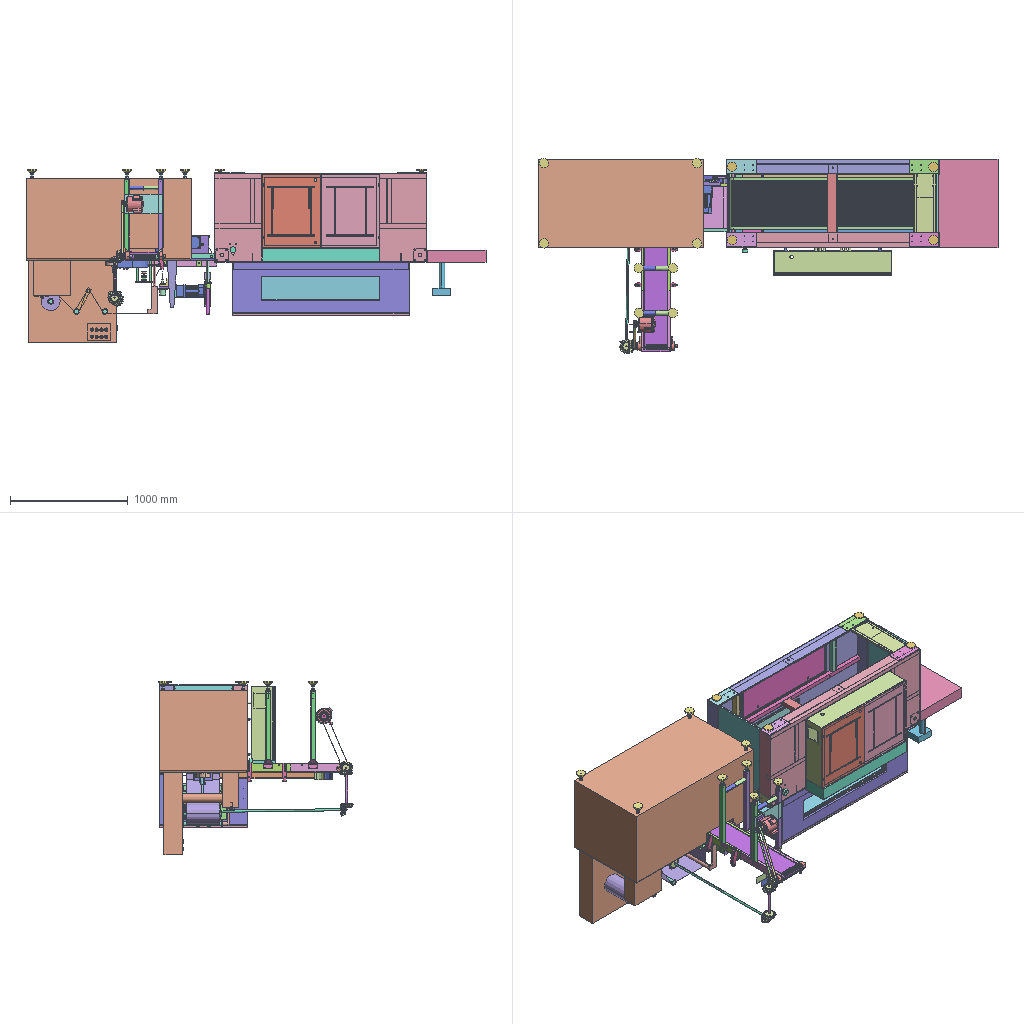Assembly | STEP file | 127 different items | 196 placed | box 3903 x 1652 x 1470 mm
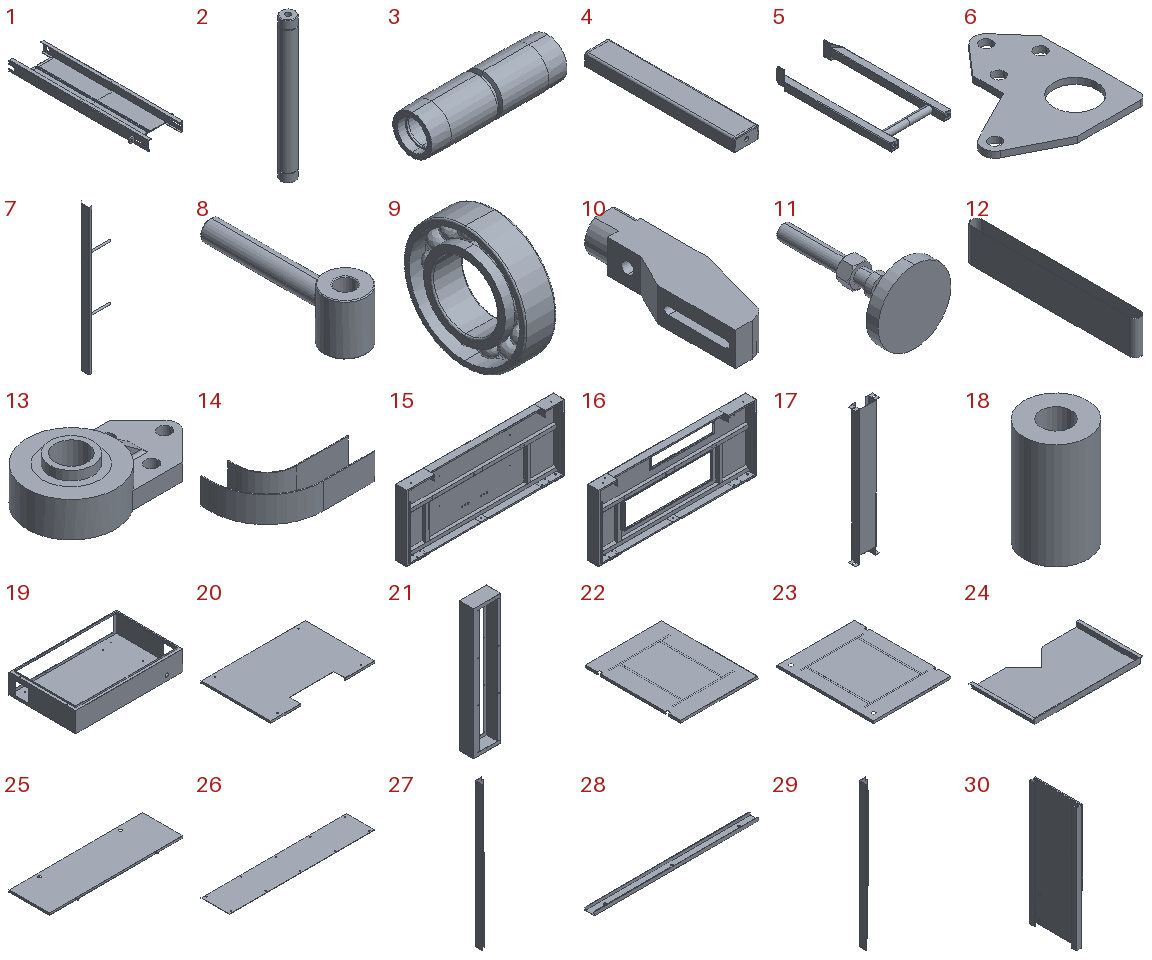Parts list (item | name | quantity | parent item | size | volume):
1 | MM-P41130-01_1 | x1 | - | 314 x 1000 x 70 mm | 800616 mm3
2 | MM-P46715-03_1 | x1 | - | 25 x 25 x 246 mm | 117700 mm3
3 | MM-P46715-04_1 | x1 | - | 215 x 64 x 64 mm | 333247 mm3
4 | MM-P46715-05_1 | x2 | - | 40 x 245 x 20 mm | 40958 mm3
5 | MM-P46715-07_1 | x2 | - | 334.243 x 661.5 x 80 mm | 460101 mm3
6 | MM-P46715-11_1 | x1 | - | 103 x 112 x 5 mm | 30189 mm3
7 | MM-P41130-12_1 | x2 | - | 151.5 x 53.167 x 800 mm | 109265 mm3
8 | M10-120_1 | x2 | - | 25 x 92.5 x 30 mm | 19534 mm3
9 | 6005-2Z_1 | x2 | - | 12 x 47 x 47 mm | 9163 mm3
10 | - | x4 | - | 44.5 x 151 x 30 mm | 132729 mm3
11 | - | x8 | - | 80 x 144 x 80 mm | 131101 mm3
12 | MM-P41130-13_1 | x1 | - | 67 x 999.5 x 200 mm | 621232 mm3
13 | UCFB205_1 | x2 | - | 116 x 68 x 34 mm | 110392 mm3
14 | - | x1 | - | 252 x 152 x 60 mm | 71299 mm3
15 | - | x1 | - | 1800 x 145 x 755 mm | 5256962 mm3
16 | - | x1 | - | 1800 x 145 x 755 mm | 4684441 mm3
17 | - | x1 | - | 120 x 40 x 664 mm | 146043 mm3
18 | - | x4 | - | 18 x 18 x 30 mm | 5932 mm3
19 | - | x1 | - | 1000 x 625 x 230.5 mm | 1788128 mm3
20 | - | x1 | - | 750 x 500 x 15 mm | 567742 mm3
21 | - | x1 | - | 210 x 110 x 1000 mm | 594029 mm3
22 | - | x1 | - | 508 x 622 x 18 mm | 582197 mm3
23 | - | x1 | - | 498 x 622 x 16 mm | 475643 mm3
24 | - | x1 | - | 316 x 180 x 15 mm | 94868 mm3
25 | - | x1 | - | 998 x 313 x 16 mm | 527029 mm3
26 | - | x1 | - | 718 x 138 x 1.5 mm | 148331 mm3
27 | - | x1 | - | 73.2 x 96 x 1315 mm | 258859 mm3
28 | - | x2 | - | 492 x 27 x 10 mm | 32318 mm3
29 | - | x1 | - | 73.2 x 96 x 1315 mm | 258859 mm3
30 | - | x1 | - | 25 x 190 x 500 mm | 670860 mm3
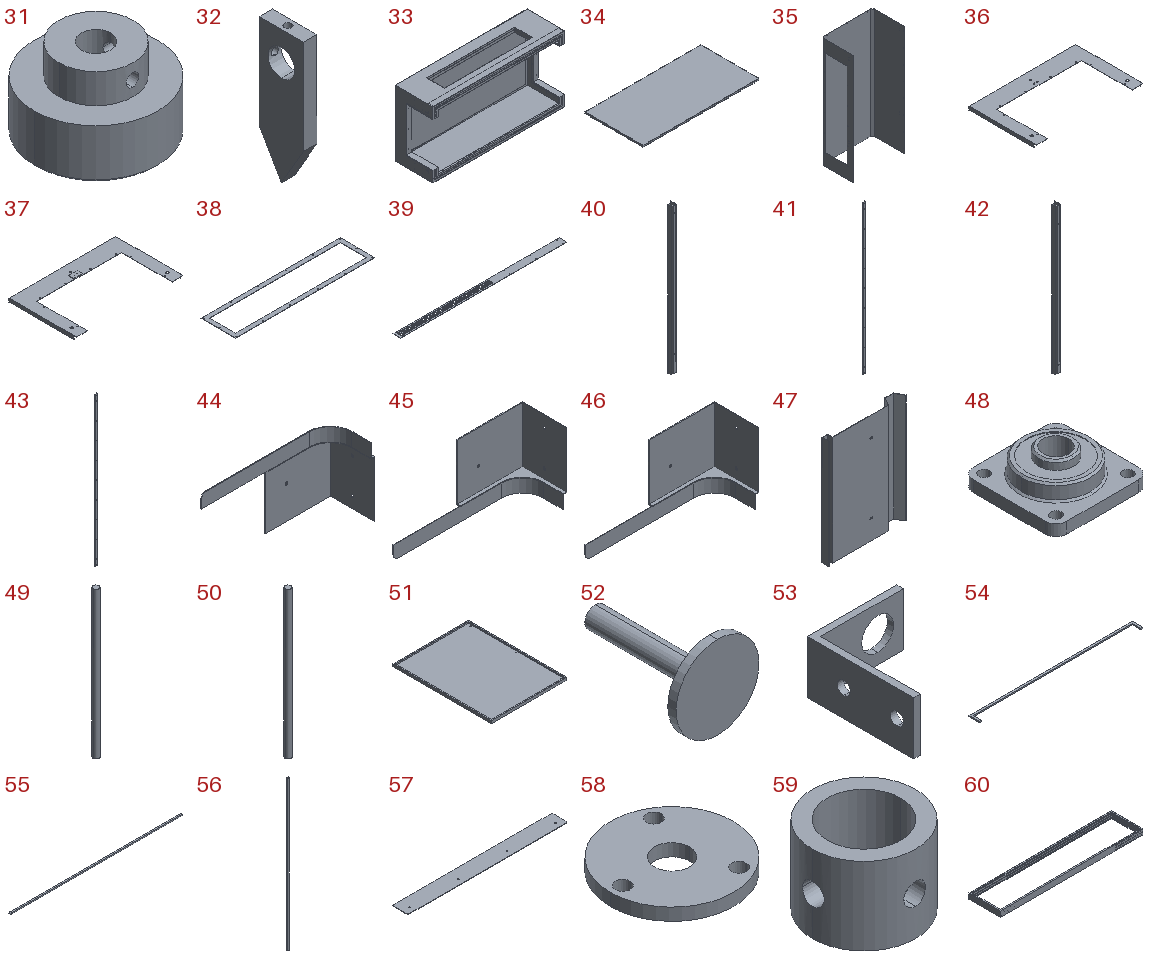31 | - | x1 | - | 50 x 50 x 32 mm | 44461 mm3
32 | - | x1 | - | 6 x 20 x 60 mm | 5382 mm3
33 | - | x1 | - | 1500 x 430 x 750 mm | 6110205 mm3
34 | - | x1 | - | 1500 x 750 x 20 mm | 1901997 mm3
35 | - | x1 | - | 628 x 396 x 1370 mm | 1949197 mm3
36 | - | x1 | - | 632 x 399.5 x 22.5 mm | 152413 mm3
37 | - | x1 | - | 632 x 399.5 x 23 mm | 156800 mm3
38 | - | x1 | - | 1064 x 264 x 2 mm | 161000 mm3
39 | - | x2 | - | 1280 x 60 x 1.5 mm | 89815 mm3
40 | - | x1 | - | 51.2 x 55 x 1530 mm | 316686 mm3
41 | - | x1 | - | 20 x 8 x 1620 mm | 65186 mm3
42 | - | x1 | - | 51.2 x 55 x 1530 mm | 316686 mm3
43 | - | x1 | - | 20 x 8 x 1620 mm | 65186 mm3
44 | - | x2 | - | 301.5 x 102 x 158 mm | 67738 mm3
45 | - | x1 | - | 301.5 x 102 x 158 mm | 67738 mm3
46 | - | x1 | - | 301.5 x 102 x 158 mm | 67738 mm3
47 | - | x1 | - | 281.999 x 34.5 x 390 mm | 208043 mm3
48 | UCF206_1 | x4 | - | 108 x 108 x 40.2 mm | 215781 mm3
49 | - | x1 | - | 30 x 30 x 742 mm | 519728 mm3
50 | - | x1 | - | 30 x 30 x 742 mm | 521298 mm3
51 | - | x2 | - | 498 x 650 x 17.5 mm | 560596 mm3
52 | - | x4 | - | 80 x 118 x 80 mm | 97023 mm3
53 | - | x4 | - | 42 x 50 x 25 mm | 5975 mm3
54 | - | x2 | - | 1458 x 94 x 10 mm | 289800 mm3
55 | - | x2 | - | 1620 x 17.6 x 10 mm | 284365 mm3
56 | - | x2 | - | 14 x 14 x 1400 mm | 203252 mm3
57 | - | x2 | - | 820 x 80 x 2 mm | 130931 mm3
58 | - | x2 | - | 50 x 50 x 5 mm | 8602 mm3
59 | - | x4 | - | 20 x 20 x 15 mm | 2256 mm3
60 | - | x1 | - | 1025 x 225 x 40 mm | 726960 mm3
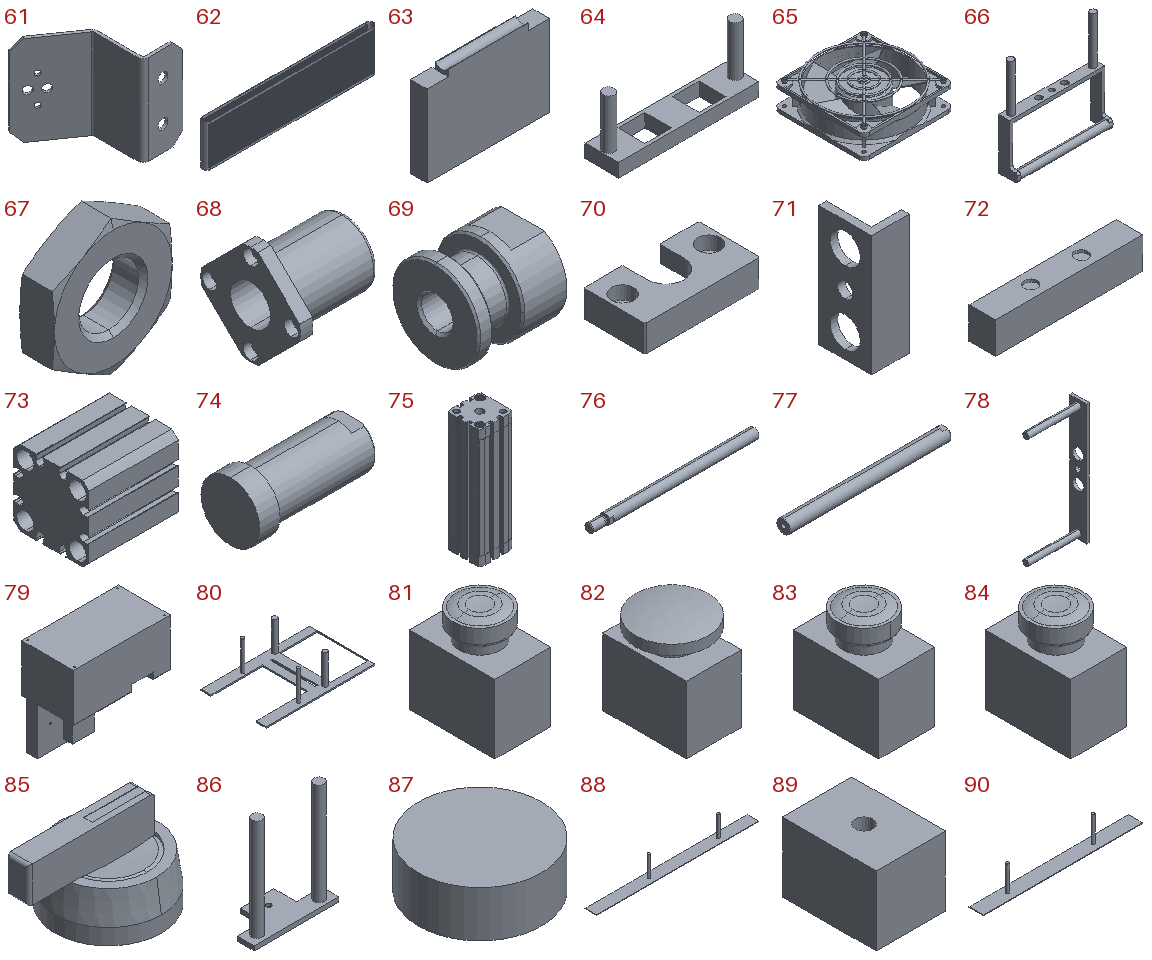61 | - | x1 | - | 44.575 x 43.436 x 45 mm | 4767 mm3
62 | - | x1 | - | 1763 x 82 x 434 mm | 1814355 mm3
63 | - | x1 | - | 750 x 100 x 540 mm | 33368808 mm3
64 | - | x1 | - | 620 x 150 x 280 mm | 4744618 mm3
65 | - | x2 | - | 122 x 122 x 36 mm | 116866 mm3
66 | - | x1 | in 214048b-01-45-00_asm_1 | 440 x 88 x 456 mm | 1386399 mm3
67 | HI_DIN-439-B - M10x1.25(F)_9-a_1_2 | x2 | in ADN-40-150-A-P-A-a_1_2, ADN-40-150-A-P-A-a_1-1_1 | 17 x 5 x 19.63 mm | 939.612 mm3
68 | LHFSF25-2.15-02-02-a_2 | x4 | in 216059B-02-40-00_2 | 59 x 62 x 62 mm | 52716 mm3
69 | FJCL10-1_25-8-a_2 | x2 | in 216059B-02-40-00_2 | 24 x 24 x 24 mm | 7197 mm3
70 | HLRA16-a_2 | x2 | in 216059B-02-40-00_2 | 56 x 30 x 13 mm | 14203 mm3
71 | - | x1 | in 216059B-02-40-00_2 | 50 x 70 x 160 mm | 147726 mm3
72 | - | x2 | in 216059B-02-40-00_2 | 280 x 50 x 60 mm | 835091 mm3
73 | _MSCCN25-15_c_1 | x1 | in MSCCN25-15_1 | 47.5 x 40 x 40 mm | 56452 mm3
74 | _MSCCN25-15_rod_1 | x1 | in MSCCN25-15_1 | 30 x 14.4 x 14.4 mm | 3377 mm3
75 | HI_536288 ADN-150P-----(Z)_1-a_1_1 | x1 | in ADN-40-150-A-P-A-a_1-1_1 | 54.5 x 54.5 x 195 mm | 304101 mm3
76 | HI_536288 ADN-150P0----(KS)_1-a_1_2 | x1 | in ADN-40-150-A-P-A-a_1-1_1 | 193.7 x 12 x 12 mm | 21128 mm3
77 | VFJC25-300-M10-SC290-qwwq-a_2 | x2 | - | 300 x 25 x 25 mm | 145438 mm3
78 | - | x1 | - | 200 x 60 x 440 mm | 380176 mm3
79 | - | x1 | - | 1400 x 750 x 1396 mm | 760190191 mm3
80 | - | x1 | - | 800 x 480 x 230 mm | 2020030 mm3
81 | ZBE-101-Y-1_1 | x1 | - | 30 x 46 x 53.196 mm | 59289 mm3
82 | ZBE-101-STOP-1_1 | x2 | - | 40 x 46 x 52.3 mm | 62411 mm3
83 | ZBE-101-R-1_1 | x1 | - | 30 x 46 x 53.196 mm | 59289 mm3
84 | ZBE-101-G-1_1 | x7 | - | 30 x 46 x 53.196 mm | 59289 mm3
85 | LAY8_1-1_1 | x1 | - | 39.873 x 29.5 x 22.9 mm | 10327 mm3
86 | - | x1 | - | 150 x 70 x 188 mm | 146525 mm3
87 | - | x1 | - | 40 x 40 x 23 mm | 20263 mm3
88 | - | x1 | - | 700 x 50 x 93 mm | 84294 mm3
89 | - | x4 | - | 40 x 54 x 40 mm | 83258 mm3
90 | - | x1 | - | 560 x 50 x 93 mm | 70294 mm3
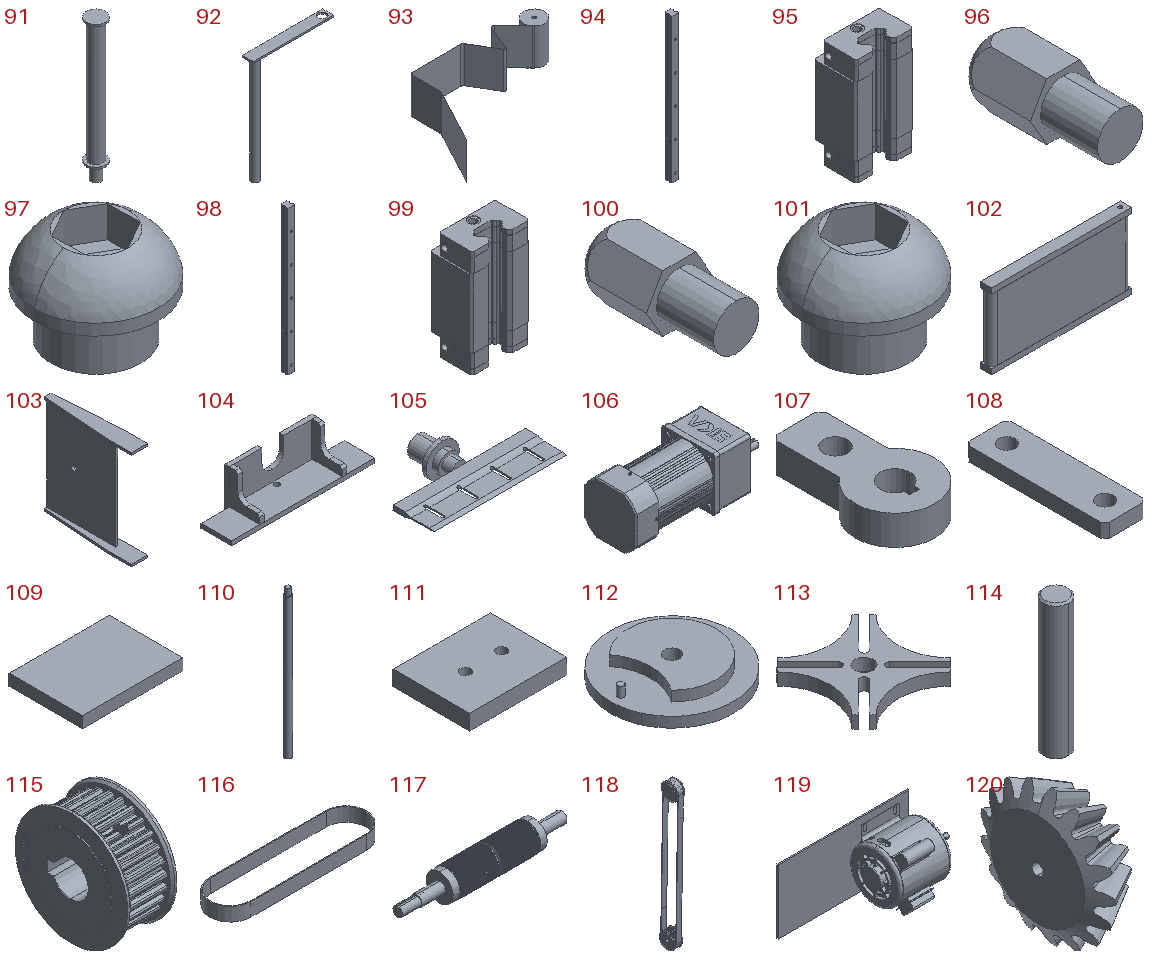91 | JUANZHOU_1 | x3 | - | 50 x 50 x 370 mm | 364990 mm3
92 | - | x1 | - | 240 x 32 x 325 mm | 157588 mm3
93 | - | x1 | - | 1160 x 667.187 x 280 mm | 5746946 mm3
94 | - | x1 | - | 15 x 15 x 300 mm | 55463 mm3
95 | - | x1 | - | 34 x 23.7 x 61.4 mm | 36598 mm3
96 | - | x1 | - | 5.774 x 12.16 x 5 mm | 199.597 mm3
97 | - | x1 | - | 5.5 x 5.5 x 4.2 mm | 58.227 mm3
98 | - | x1 | - | 15 x 15 x 300 mm | 55463 mm3
99 | - | x1 | - | 34 x 23.7 x 61.4 mm | 36598 mm3
100 | - | x1 | - | 5.774 x 12.16 x 5 mm | 199.597 mm3
101 | - | x1 | - | 5.5 x 5.5 x 4.2 mm | 58.227 mm3
102 | - | x1 | - | 760 x 60 x 410 mm | 18296796 mm3
103 | - | x1 | - | 70 x 400 x 430 mm | 1666858 mm3
104 | - | x1 | - | 330 x 80 x 90 mm | 438268 mm3
105 | - | x1 | - | 320 x 200 x 80 mm | 390081 mm3
106 | - | x2 | - | 277 x 108.652 x 108.652 mm | 2253105 mm3
107 | - | x1 | - | 40 x 70 x 15 mm | 25956 mm3
108 | - | x1 | - | 30 x 100 x 10 mm | 27558 mm3
109 | - | x1 | - | 150 x 110 x 17 mm | 280500 mm3
110 | - | x1 | - | 20 x 20 x 460 mm | 141681 mm3
111 | - | x1 | - | 190 x 150 x 30 mm | 836150 mm3
112 | - | x1 | - | 120 x 120 x 20 mm | 158754 mm3
113 | - | x1 | - | 79.917 x 79.917 x 10 mm | 31022 mm3
114 | - | x1 | - | 15 x 15 x 80 mm | 14092 mm3
115 | - | x2 | - | 22 x 48 x 48 mm | 27125 mm3
116 | - | x1 | - | 173.39 x 45.75 x 15 mm | 5938 mm3
117 | MM-P46715-02_1 | x1 | in Modified main assembly | 375.959 x 63.996 x 63.999 mm | 524542 mm3
118 | _X2_51434EF6_X0_21_1 | x1 | in Modified main assembly | 29.173 x 69.582 x 540.649 mm | 150138 mm3
119 | _X2_51434EF6_X0_22_1 | x1 | in Modified main assembly | 358.567 x 145.946 x 163 mm | 1839939 mm3
120 | Bevel gear 17×2 | x6 | in Modified main assembly | 38.391 x 112.113 x 112.556 mm | 206962 mm3
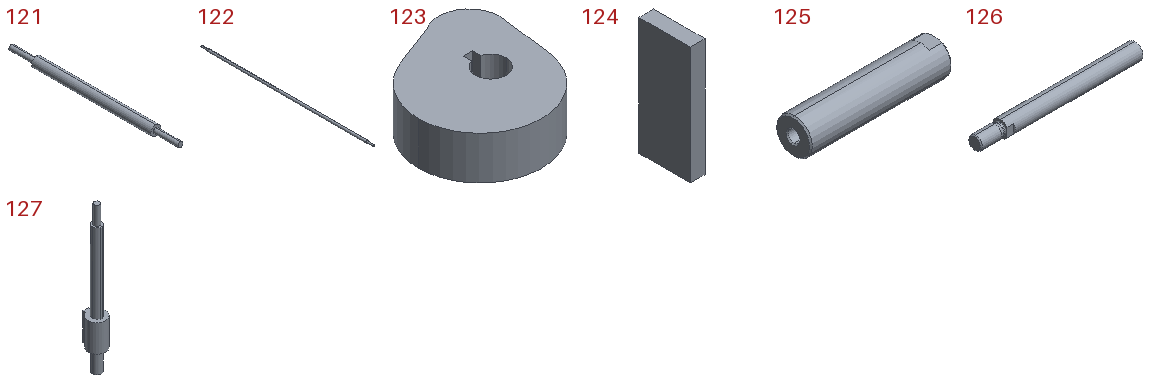121 | Fixed long shaft | x1 | in Modified main assembly | 19.77 x 340 x 19.77 mm | 81528 mm3
122 | Bevel gear fixed shaft | x1 | in Modified main assembly | 18 x 1200 x 18 mm | 287770 mm3
123 | Disc cam | x1 | in Modified main assembly | 105.129 x 114.018 x 35 mm | 298782 mm3
124 | Part 1 | x1 | in Modified main assembly | 20 x 70 x 160 mm | 224000 mm3
125 | Part 2 | x2 | in Modified main assembly | 100 x 25 x 25 mm | 47263 mm3
126 | Part 4 | x1 | in Modified main assembly | 119 x 12 x 12 mm | 12679 mm3
127 | Camshaft | x1 | in Modified main assembly | 38.228 x 43.828 x 320 mm | 147567 mm3
Placements (level | parent | child | x y z in mm | rotation matrix by rows):
1 | Modified main assembly | subassembly 2 | -1135.176 -5611.395 2452.198 | 1 0 0 0 1 0 0 0 1
2 | subassembly 2 | MM-P41130-01_1 | 910.011 5927.051 -736.46 | -1 0 0 0 -1 0 0 0 1
2 | subassembly 2 | MM-P46715-03_1 | 910.011 6389.551 -736.5 | 0 0 1 -0.5368 -0.8437 0 0.8437 -0.5368 0
2 | subassembly 2 | MM-P46715-04_1 | 910.011 6389.551 -736.5 | -1 0 0 0 0.8554 -0.5179 0 -0.5179 -0.8554
2 | subassembly 2 | MM-P46715-05_1 | 910.011 5427.051 -721.5 | 0 1 0 1 0 0 0 0 -1
2 | subassembly 2 | MM-P46715-05_1 | 910.011 6427.051 -721.5 | 0 1 0 1 0 0 0 0 -1
2 | subassembly 2 | MM-P46715-07_1 | 910.011 5737.051 -80.0 | -1 0 0 0 0 -1 0 -1 -0
2 | subassembly 2 | MM-P46715-07_1 | 910.011 6117.051 -80.0 | -1 0 0 0 0 -1 0 -1 0
2 | subassembly 2 | MM-P46715-11_1 | 1040.011 5457.051 -736.5 | 0 0 -1 0 1 0 1 0 0
2 | subassembly 2 | MM-P41130-12_1 | 878.511 6127.051 -825.0 | -1 0 0 0 0 -1 0 -1 0
2 | subassembly 2 | MM-P41130-12_1 | 941.511 6127.051 -825.0 | 1 0 0 0 0 1 0 -1 -0
2 | subassembly 2 | M10-120_1 | 785.011 6389.551 -736.5 | 0 0 -1 0 -1 0 -1 0 -0
2 | subassembly 2 | M10-120_1 | 1067.373 6389.551 -736.5 | 0 0 -1 0 -1 0 -1 0 -0
2 | subassembly 2 | 6005-2Z_1 | 808.511 6389.551 -736.5 | -1 0 0 0 -0.2495 0.9684 0 0.9684 0.2495
2 | subassembly 2 | 6005-2Z_1 | 1011.511 6389.551 -736.5 | -1 0 0 0 -0.2495 0.9684 0 0.9684 0.2495
2 | subassembly 2 | subassembly 3 | 762.761 6277.051 -772.0 | -1 0 0 0 0 -1 0 -1 0
2 | subassembly 2 | subassembly 4 | 1055.011 5737.051 -0.0 | 0.1728 0 0.985 -0.985 0 0.1728 0 -1 -0
2 | subassembly 2 | subassembly 4 | 1055.011 6117.051 -0.0 | 0.2654 0 0.9641 -0.9641 0 0.2654 0 -1 -0
2 | subassembly 2 | subassembly 4 | 765.011 6117.051 -0.0 | -0.5406 0 -0.8413 0.8413 0 -0.5406 0 -1 -0
2 | subassembly 2 | subassembly 4 | 765.011 5737.051 -0.0 | -0.8402 0 -0.5422 0.5422 0 -0.8402 0 -1 -0
2 | subassembly 2 | subassembly 3 | 1057.261 6277.051 -772.0 | 1 0 0 0 0 1 0 -1 -0
2 | subassembly 2 | MM-P41130-13_1 | 910.011 6404.551 -720 | 0 0 1 0 1 0 -1 0 0
2 | subassembly 2 | subassembly 3 | 762.761 5977.051 -772.0 | -1 0 0 0 0 -1 0 -1 0
2 | subassembly 2 | subassembly 3 | 1057.261 5977.051 -772.0 | 1 0 0 0 0 1 0 -1 0
2 | subassembly 2 | UCFB205_1 | 1040.011 5457.051 -736.5 | 0 0 1 1 0 0 0 1 0
2 | subassembly 2 | UCFB205_1 | 785.011 5457.051 -736.5 | 0 0 -1 1 0 0 0 -1 0
2 | subassembly 2 | subassembly 5 | 910.011 5607.051 -773.5 | -1 0 0 0 1 0 0 0 -1
1 | Modified main assembly | subassembly 6 | 1501.804 1134.386 1912.405 | -1 0 0 0 0 -1 0 -1 -0
2 | subassembly 6 | subassembly 7 | 225.469 -504.793 453.729 | -1 0 0 0 0 1 0 1 0
2 | subassembly 6 | subassembly 8 | 225.469 -504.793 -296.271 | 1 0 0 0 0 1 0 -1 0
2 | subassembly 6 | subassembly 9 | 229.469 -59.792 79.729 | -1 0 0 0 1 0 0 0 -1
2 | subassembly 6 | subassembly 10 | -174.531 80.207 483.729 | 0.9237 0.383 0 0.383 -0.9237 0 0 0 -1
2 | subassembly 6 | subassembly 10 | 625.469 -219.792 483.729 | 0.9237 0.383 0 0.383 -0.9237 0 0 0 -1
2 | subassembly 6 | subassembly 10 | 625.469 80.207 483.729 | 0.9237 0.383 0 0.383 -0.9237 0 0 0 -1
2 | subassembly 6 | subassembly 10 | -174.531 -219.792 483.729 | 0.9237 0.383 0 0.383 -0.9237 0 0 0 -1
2 | subassembly 6 | subassembly 11 | 225.469 -182.292 483.729 | 1 0 0 0 1 0 0 0 1
2 | subassembly 6 | subassembly 12 | 225.469 -169.792 491.729 | 1 0 0 0 1 0 0 0 1
2 | subassembly 6 | subassembly 13 | 225.469 185.208 587.229 | 0 0 1 0 1 0 -1 0 0
2 | subassembly 6 | subassembly 14 | -274.531 -494.793 668.729 | 1 0 0 0 1 0 0 0 1
2 | subassembly 6 | subassembly 15 | 476.469 -183.792 670.729 | 1 0 0 0 1 0 0 0 1
2 | subassembly 6 | subassembly 16 | 477.469 -294.543 685.529 | 1 0 0 0 1 0 0 0 1
2 | subassembly 6 | subassembly 17 | 225.469 -254.792 -292.271 | -1 0 0 0 1 0 0 0 -1
2 | subassembly 6 | subassembly 18 | 400.469 105.207 -294.271 | 1 0 0 0 1 0 0 0 1
2 | subassembly 6 | subassembly 19 | 175.469 174.407 -171.771 | 0 0 -1 1 0 0 0 -1 0
2 | subassembly 6 | subassembly 20 | 955.469 548.207 78.729 | 0 1 0 0 0 -1 -1 0 0
2 | subassembly 6 | subassembly 20 | -504.531 548.207 78.729 | 0 1 0 0 0 -1 -1 0 0
2 | subassembly 6 | subassembly 21 | -731.989 174.407 329.229 | 0 0 1 1 0 0 0 1 0
2 | subassembly 6 | subassembly 22 | -557.531 -489.793 -171.271 | 0 -1 0 1 0 0 0 0 1
2 | subassembly 6 | subassembly 23 | 970.469 142.208 493.729 | -0.9237 -0.383 0 -0.383 0.9237 0 0 0 -1
2 | subassembly 6 | subassembly 24 | 970.469 129.208 457.729 | 0 -1 0 0 0 -1 1 0 0
2 | subassembly 6 | subassembly 25 | 225.469 248.208 78.729 | 1 0 0 0 1 0 0 0 1
2 | subassembly 6 | subassembly 26 | 225.469 678.207 78.729 | 1 0 0 0 0 1 0 -1 0
2 | subassembly 6 | subassembly 27 | 225.469 447.707 78.729 | 0 0 1 0 1 0 -1 0 0
2 | subassembly 6 | subassembly 28 | -444.531 448.957 78.729 | 0 0 -1 0 1 0 1 0 0
2 | subassembly 6 | subassembly 29 | 895.469 448.957 2029.668 | 0 0 1 0 1 0 -1 0 0
2 | subassembly 6 | subassembly 30 | 225.469 468.207 390.229 | 1 0 0 0 1 0 0 0 1
2 | subassembly 6 | subassembly 31 | 175.469 245.208 -202.471 | -1 0 0 0 0 -1 0 -1 0
2 | subassembly 6 | subassembly 31 | 175.469 245.208 359.929 | -1 0 0 0 0 -1 0 -1 0
2 | subassembly 6 | subassembly 32 | -539.531 174.407 276.729 | 0 0 -1 0 1 0 1 0 0
2 | subassembly 6 | subassembly 33 | 225.469 209.407 285.529 | 0 0 -1 0 1 0 1 0 0
2 | subassembly 6 | subassembly 34 | 53.011 174.407 -119.271 | 0 0 1 0 1 0 -1 0 0
2 | subassembly 6 | subassembly 35 | 818.011 209.407 -128.071 | 0 0 1 0 1 0 -1 0 0
2 | subassembly 6 | subassembly 36 | 976.969 145.208 -168.271 | 1 0 0 0 1 0 0 0 1
2 | subassembly 6 | subassembly 36 | -526.031 145.208 325.729 | -1 0 0 0 1 0 0 0 -1
2 | subassembly 6 | subassembly 37 | 976.969 145.208 668.271 | 1 0 0 0 1 0 0 0 1
2 | subassembly 6 | subassembly 38 | -526.031 145.208 -510.813 | -1 0 0 0 1 0 0 0 -1
2 | subassembly 6 | subassembly 39 | 816.969 182.208 79.729 | 1 0 0 0 1 0 0 0 1
2 | subassembly 6 | UCF206_1 | 1065.969 185.708 451.729 | -1 0 0 0 1 0 0 0 -1
2 | subassembly 6 | UCF206_1 | 1065.969 185.708 -294.271 | 0 -1 0 1 0 0 0 0 1
2 | subassembly 6 | UCF206_1 | -615.031 185.708 -294.271 | 1 0 0 0 1 0 0 0 1
2 | subassembly 6 | UCF206_1 | -615.031 185.708 451.729 | -1 0 0 0 1 0 0 0 -1
2 | subassembly 6 | subassembly 40 | -615.031 185.708 78.729 | -0.717 -0.6971 0 0.6971 -0.717 0 0 0 1
2 | subassembly 6 | subassembly 41 | 1065.969 185.708 78.729 | 0.644 -0.765 0 0.765 0.644 0 0 0 1
2 | subassembly 6 | subassembly 42 | -672.031 -179.792 78.729 | 0 0 1 0 1 0 -1 0 0
2 | subassembly 6 | subassembly 42 | 1122.969 -179.792 78.729 | 0 0 -1 0 1 0 1 0 0
2 | subassembly 6 | subassembly 43 | 1080.469 -539.793 -231.271 | -0.6355 0 0.7721 0 1 0 -0.7721 0 -0.6355
2 | subassembly 6 | subassembly 43 | 1080.469 -539.793 388.729 | 1 0 0 0 1 0 0 0 1
2 | subassembly 6 | subassembly 43 | -629.531 -539.793 -231.271 | 1 0 0 0 1 0 0 0 1
2 | subassembly 6 | subassembly 43 | -629.531 -539.793 388.729 | 1 0 0 0 1 0 0 0 1
2 | subassembly 6 | subassembly 44 | -81.531 309.707 -234.071 | 0 -1 0 0 0 -1 1 0 0
2 | subassembly 6 | subassembly 44 | -81.531 309.707 391.529 | 0 -1 0 0 0 1 -1 0 0
2 | subassembly 6 | subassembly 44 | 818.469 309.707 -234.071 | 0 -1 0 0 0 -1 1 0 0
2 | subassembly 6 | subassembly 44 | 818.469 309.707 391.529 | 0 -1 0 0 0 1 -1 0 0
2 | subassembly 6 | subassembly 45 | -485.531 255.208 338.729 | 1 0 0 0 0 -1 0 1 0
2 | subassembly 6 | subassembly 45 | -485.531 245.208 -181.271 | 1 0 0 0 0 1 0 -1 0
2 | subassembly 6 | subassembly 46 | -584.531 210.607 294.329 | 1 0 0 0 0 1 0 -1 0
2 | subassembly 6 | subassembly 46 | -584.531 210.607 -119.271 | 1 0 0 0 0 1 0 -1 0
2 | subassembly 6 | subassembly 47 | 66.469 309.707 361.529 | 0 0 -1 0.9202 0.3914 0 0.3914 -0.9202 0
2 | subassembly 6 | subassembly 47 | 66.469 309.707 -204.071 | 0 0 -1 0.6674 -0.7447 0 -0.7447 -0.6674 0
2 | subassembly 6 | subassembly 48 | 381.469 314.717 -190.182 | -1 0 0 0 0.7447 0.6674 0 0.6674 -0.7447
2 | subassembly 6 | subassembly 48 | 381.469 310.195 347.609 | -1 0 0 0 0.3914 -0.9202 0 -0.9202 -0.3914
2 | subassembly 6 | subassembly 49 | -529.531 309.207 -204.271 | 0 0 1 0.5 -0.866 0 0.866 0.5 0
2 | subassembly 6 | subassembly 49 | -529.531 309.207 361.729 | 0 0 1 0.5 -0.866 0 0.866 0.5 0
2 | subassembly 6 | subassembly 50 | -89.031 309.707 -204.071 | 0 0 1 0 1 0 -1 0 0
2 | subassembly 6 | subassembly 50 | -455.831 309.707 -204.071 | 0 0 1 0 1 0 -1 0 0
2 | subassembly 6 | subassembly 50 | -455.831 309.707 361.529 | 0 0 1 0 1 0 -1 0 0
2 | subassembly 6 | subassembly 50 | -89.031 309.707 361.529 | 0 0 -1 -0.9242 -0.3818 0 -0.3818 0.9242 0
2 | subassembly 6 | subassembly 51 | -287.031 355.707 392.229 | 1 0 0 0 1 0 0 0 1
2 | subassembly 6 | subassembly 52 | -463.331 580.207 56.229 | 0 1 0 -1 0 0 0 0 1
2 | subassembly 6 | subassembly 53 | -615.031 185.708 78.729 | 1 0 0 0 1 0 0 0 1
2 | subassembly 6 | subassembly 54 | -1176.031 197.208 78.729 | 0 0 1 0 1 0 -1 0 0
2 | subassembly 6 | subassembly 55 | -799.531 527.207 78.729 | 0 1 0 0 0 -1 -1 0 -0
2 | subassembly 6 | subassembly 56 | -799.531 495.207 -41.271 | 0 1 0 0 0 1 1 0 0
2 | subassembly 6 | subassembly 56 | -799.531 495.207 198.729 | 0 1 0 0 0 1 1 0 0
1 | Modified main assembly | subassembly 57 | -458.134 1171.525 630.197 | 1 0 0 0 1 0 0 0 1
2 | subassembly 57 | 214048b-01-45-00_asm_1 | 322.969 -115.868 832.0 | 0 0 1 -1 0 0 0 -1 0
3 | 214048b-01-45-00_asm_1 | subassembly 58 | -0.0 16.0 -0.0 | 1 0 0 0 0 -1 0 1 0
2 | subassembly 57 | 216059B-02-40-00_2 | 43.29 249.132 1025.139 | 0 -1 0 0 0 -1 1 0 -0
3 | 216059B-02-40-00_2 | ADN-40-150-A-P-A-a_1_2 | -8.139 -49.678 365.0 | 1 0 0 0 0 -1 0 1 0
4 | ADN-40-150-A-P-A-a_1_2 | HI_DIN-439-B - M10x1.25(F)_9-a_1_2 | -0.0 -0.0 15.1 | 1 0 0 0 0 -1 0 1 0
3 | 216059B-02-40-00_2 | LHFSF25-2.15-02-02-a_2 | -8.139 -67.678 413.0 | 0 -0.7071 0.7071 1 0 0 0 0.7071 0.7071
3 | 216059B-02-40-00_2 | LHFSF25-2.15-02-02-a_2 | -8.139 -67.678 317.0 | 0 -0.7071 0.7071 1 0 0 0 0.7071 0.7071
3 | 216059B-02-40-00_2 | FJCL10-1_25-8-a_2 | -8.139 -88.778 365.0 | 0 0.8298 -0.558 1 0 0 0 -0.558 -0.8298
3 | 216059B-02-40-00_2 | HLRA16-a_2 | -8.139 -89.778 365.0 | 0 1 0 0 0 1 1 0 0
3 | 216059B-02-40-00_2 | subassembly 59 | 16.861 -49.678 365.0 | 0 -1 0 1 0 0 0 0 1
3 | 216059B-02-40-00_2 | subassembly 60 | -8.139 -144.306 365.0 | 0 -1 0 0 0 1 -1 0 0
2 | subassembly 57 | MSCCN25-15_1 | 232.969 -286.708 872.0 | 0 0 -1 0 1 0 1 0 0
3 | MSCCN25-15_1 | _MSCCN25-15_c_1 | -0.0 -0.0 -0.0 | 1 0 0 0 1 0 0 0 1
3 | MSCCN25-15_1 | _MSCCN25-15_rod_1 | 32.274 -0.0 -0.0 | 1 0 0 0 0.5537 -0.8327 0 0.8327 0.5537
2 | subassembly 57 | subassembly 61 | 783.22 -480.868 802.322 | 1 0 0 0 0 1 0 -1 0
3 | subassembly 61 | ADN-40-150-A-P-A-a_1-1_1 | -8.139 -49.678 365.0 | 1 0 0 0 0 -1 0 1 0
4 | ADN-40-150-A-P-A-a_1-1_1 | HI_536288 ADN-150P-----(Z)_1-a_1_1 | -0.0 -0.0 -0.0 | 1 0 0 0 1 0 0 0 1
4 | ADN-40-150-A-P-A-a_1-1_1 | HI_536288 ADN-150P0----(KS)_1-a_1_2 | -0.0 -0.0 -0.0 | 0 0.957 0.2901 0 0.2901 -0.957 -1 0 0
4 | ADN-40-150-A-P-A-a_1-1_1 | HI_DIN-439-B - M10x1.25(F)_9-a_1_2 | -0.0 -0.0 15.1 | 1 0 0 0 0 -1 0 1 0
3 | subassembly 61 | LHFSF25-2.15-02-02-a_2 | -8.139 -67.678 413.0 | 0 -0.7071 0.7071 1 0 0 0 0.7071 0.7071
3 | subassembly 61 | LHFSF25-2.15-02-02-a_2 | -8.139 -67.678 317.0 | 0 -0.7071 0.7071 1 0 0 0 0.7071 0.7071
3 | subassembly 61 | FJCL10-1_25-8-a_2 | -8.139 -88.778 365.0 | 0 0.8298 -0.558 1 0 0 0 -0.558 -0.8298
3 | subassembly 61 | HLRA16-a_2 | -8.139 -89.778 365.0 | 0 1 0 0 0 1 1 0 0
3 | subassembly 61 | VFJC25-300-M10-SC290-qwwq-a_2 | -8.139 -89.306 317.0 | 0 0.3448 0.9387 1 0 0 0 0.9387 -0.3448
3 | subassembly 61 | VFJC25-300-M10-SC290-qwwq-a_2 | -8.139 -89.306 413.0 | 0 0.9001 0.4357 1 0 0 0 0.4357 -0.9001
3 | subassembly 61 | subassembly 62 | 21.861 -49.678 365.0 | 0 -1 0 1 0 0 0 0 1
3 | subassembly 61 | subassembly 60 | -8.139 -144.306 365.0 | 0 -1 0 0 0 1 -1 0 0
2 | subassembly 57 | subassembly 63 | -67.031 -115.868 1052.0 | 1 0 0 0 1 0 0 0 1
2 | subassembly 57 | subassembly 4 | 582.969 -455.868 1822.0 | 0.9965 0 -0.08316 0.08316 0 0.9965 0 -1 -0
2 | subassembly 57 | subassembly 4 | 582.969 224.132 1822.0 | 0.9965 0 -0.08316 0.08316 0 0.9965 0 -1 -0
2 | subassembly 57 | subassembly 4 | -717.031 224.132 1822.0 | 0.9965 0 -0.08316 0.08316 0 0.9965 0 -1 -0
2 | subassembly 57 | subassembly 4 | -717.031 -455.868 1822.0 | 0.9965 0 -0.08316 0.08316 0 0.9965 0 -1 -0
2 | subassembly 57 | subassembly 64 | 452.969 -115.868 1052.0 | -1 0 0 0 -1 0 0 0 1
2 | subassembly 57 | ZBE-101-Y-1_1 | -41.866 80.382 378.086 | 0.8908 -0.4544 0 0 0 -1 0.4544 0.8908 0
2 | subassembly 57 | ZBE-101-STOP-1_1 | -23.781 131.027 652.39 | 0 0 1 0.2727 -0.9621 0 0.9621 0.2727 0
2 | subassembly 57 | ZBE-101-R-1_1 | -40.032 80.382 476.94 | 0.965 -0.2621 0 0 0 -1 0.2621 0.965 0
2 | subassembly 57 | ZBE-101-G-1_1 | 52.354 80.382 355.244 | 0.9539 0.3001 0 0 0 -1 -0.3001 0.9539 0
2 | subassembly 57 | LAY8_1-1_1 | -670.304 -238.633 773.0 | -0.3306 0.9438 0 0.9438 0.3306 0 0 0 -1
2 | subassembly 57 | ZBE-101-G-1_1 | 12.354 80.382 355.244 | 0.9539 0.3001 0 0 0 -1 -0.3001 0.9539 0
2 | subassembly 57 | ZBE-101-G-1_1 | -27.646 80.382 355.244 | 0.9539 0.3001 0 0 0 -1 -0.3001 0.9539 0
2 | subassembly 57 | ZBE-101-G-1_1 | -67.646 80.382 355.244 | 0.9539 0.3001 0 0 0 -1 -0.3001 0.9539 0
2 | subassembly 57 | ZBE-101-STOP-1_1 | -546.035 -463.48 778.75 | 0.9304 -0.3666 0 -0.3666 -0.9304 0 0 0 -1
2 | subassembly 57 | ZBE-101-G-1_1 | -67.646 80.382 295.244 | 0.9539 0.3001 0 0 0 -1 -0.3001 0.9539 0
2 | subassembly 57 | ZBE-101-G-1_1 | -27.646 80.382 295.244 | 0.9539 0.3001 0 0 0 -1 -0.3001 0.9539 0
2 | subassembly 57 | ZBE-101-G-1_1 | -419.008 -297.885 774.25 | 0.9979 -0.06421 0 -0.06421 -0.9979 0 0 0 -1
2 | subassembly 57 | subassembly 65 | 232.969 -335.868 864.0 | 1 0 0 0 1 0 0 0 1
2 | subassembly 57 | subassembly 66 | 232.969 -286.708 942.274 | 1 0.001777 0 -0.001777 1 0 0 0 1
2 | subassembly 57 | subassembly 67 | 502.969 24.132 1025.0 | 1 0 0 0 0 1 0 -1 0
2 | subassembly 57 | subassembly 68 | 402.969 124.132 1025.0 | 1 0 0 0 0 -1 0 1 0
2 | subassembly 57 | subassembly 68 | 702.969 124.132 1025.0 | 1 0 0 0 0 -1 0 1 0
2 | subassembly 57 | subassembly 69 | 572.969 -255.868 1025.0 | 1 0 0 0 0 -1 0 1 0
2 | subassembly 57 | subassembly 68 | 702.969 -315.868 1025.0 | 1 0 0 0 0 -1 0 1 0
2 | subassembly 57 | subassembly 68 | 402.969 -315.868 1025.0 | 1 0 0 0 0 -1 0 1 0
2 | subassembly 57 | JUANZHOU_1 | -97.031 -105.868 616.0 | 0.8247 0.5655 0 0 0 -1 -0.5655 0.8247 0
2 | subassembly 57 | subassembly 70 | -286.031 54.132 704.335 | -0.5 -0.866 0 0 0 1 -0.866 0.5 0
2 | subassembly 57 | JUANZHOU_1 | -337.031 -110.868 616.0 | -0.001163 -1 0 0 0 -1 1 -0.001163 0
2 | subassembly 57 | JUANZHOU_1 | -557.031 -105.868 702.0 | 0.7722 0.6354 0 0 0 -1 -0.6354 0.7722 0
2 | subassembly 57 | subassembly 71 | -557.031 24.132 702.0 | -1 0 0 0 0 -1 0 -1 0
1 | Modified main assembly | subassembly 72 | 20.284 1044.76 1759.601 | 0.9993 -0.008725 0.03505 -0.03489 0.01745 0.9992 -0.00933 -0.9998 0.01714
2 | subassembly 72 | subassembly 73 | -5.972 253.662 -132.388 | 0.00933 -0.9993 -0.03489 0.9998 0.008725 0.01745 -0.01714 -0.03505 0.9992
3 | subassembly 73 | subassembly 74 | -150.0 -0.0 -0.0 | 0 0 -1 0 1 0 1 0 0
3 | subassembly 73 | subassembly 75 | 14.178 0.0 -0.0 | 0 0 1 0 1 0 -1 0 -0
3 | subassembly 73 | subassembly 76 | -17.732 5.05 -0.0 | 0 -1 0 0.866 0 0.5 -0.5 0 0.866
3 | subassembly 73 | subassembly 77 | 40.785 4.407 1.113 | 0 0 1 0.5 0.866 0 -0.866 0.5 -0
2 | subassembly 72 | subassembly 78 | -16.265 258.81 162.387 | 0.00933 -0.9993 -0.03489 0.9998 0.008725 0.01745 -0.01714 -0.03505 0.9992
3 | subassembly 78 | subassembly 79 | -150.0 -0.0 -0.0 | 0 0 -1 0 1 0 1 0 0
3 | subassembly 78 | subassembly 80 | 14.178 -0.0 -0.0 | 0 0 1 0 1 0 -1 0 -0
3 | subassembly 78 | subassembly 81 | -17.732 5.05 -0.0 | 0 -1 0 0.866 0 0.5 -0.5 0 0.866
3 | subassembly 78 | subassembly 82 | 40.785 4.407 1.113 | 0 0 1 0.5 0.866 0 -0.866 0.5 -0
2 | subassembly 72 | subassembly 83 | -20.404 47.163 -25.658 | 0.9993 0.00933 -0.03489 -0.008725 0.9998 0.01745 0.03505 -0.01714 0.9992
2 | subassembly 72 | subassembly 84 | -3.483 327.705 10.023 | 0.9993 0.009336 -0.03489 -0.008725 0.9998 0.01761 0.03505 -0.0173 0.9992
2 | subassembly 72 | subassembly 85 | -23.978 270.525 14.301 | -0.03489 0.00933 -0.9993 0.01745 0.9998 0.008725 0.9992 -0.01714 -0.03505
2 | subassembly 72 | subassembly 86 | -83.892 276.048 12.112 | -0.03489 0.00933 -0.9993 0.01745 0.9998 0.008725 0.9992 -0.01714 -0.03505
2 | subassembly 72 | subassembly 87 | 31.647 340.853 15.015 | -0.9993 -0.00933 -0.03489 0.008725 -0.9998 0.01745 -0.03505 0.01714 0.9992
2 | subassembly 72 | subassembly 88 | -2.644 361.151 13.463 | 0.01223 0.03399 -0.9993 0.9948 -0.1016 0.008725 -0.1012 -0.9942 -0.03505
2 | subassembly 72 | subassembly 89 | -16.932 326.849 -1.395 | 0.02757 0.02334 0.9993 -0.4427 0.8966 -0.008725 -0.8962 -0.4422 0.03505
2 | subassembly 72 | subassembly 90 | 31.647 340.853 15.015 | -0.03489 0.00933 -0.9993 0.01745 0.9998 0.008725 0.9992 -0.01714 -0.03505
2 | subassembly 72 | subassembly 91 | 328.009 44.789 25.52 | 0.2798 0.9594 -0.03489 -0.9597 0.2805 0.01745 0.02653 0.0286 0.9992
2 | subassembly 72 | subassembly 92 | 204.454 -55.69 171.94 | 1 0 0 0 1 0 0 0 1
2 | subassembly 72 | subassembly 93 | 228.5 -103.248 212.94 | -0.74 -0.6726 0 0.6726 -0.74 0 0 0 1
2 | subassembly 72 | subassembly 94 | 246.882 -55.69 212.94 | -1 -0.00059 0 0.00059 -1 0 0 0 1
2 | subassembly 72 | subassembly 87 | 176.171 -75.69 171.94 | 0 0 1 0 -1 0 1 0 -0
2 | subassembly 72 | subassembly 95 | 246.882 -55.69 211.94 | 0.9993 0.03807 0 -0.03807 0.9993 0 0 0 1
2 | subassembly 72 | subassembly 96 | 320.064 48.763 253.037 | 0.03489 -0.1098 0.9933 -0.01745 0.9937 0.1104 -0.9992 -0.02119 0.03276
2 | subassembly 72 | subassembly 96 | 249.287 -57.353 252.016 | -0.007838 0.4618 0.8869 0.005419 0.887 -0.4618 -1 0.001186 -0.009455
2 | subassembly 72 | subassembly 97 | 284.185 -3.941 241.181 | 0.5685 -0.822 -0.03489 0.8227 0.5682 0.01745 0.005483 -0.03863 0.9992
1 | Modified main assembly | MM-P46715-02_1 | -215.646 -154.343 1715.697 | 1 0 0 0 1 0 0 0 1
1 | Modified main assembly | _X2_51434EF6_X0_21_1 | -0.0 402.409 3345.443 | 1 0 0 0 -0.9135 -0.4067 0 0.4067 -0.9135
1 | Modified main assembly | _X2_51434EF6_X0_22_1 | -1059.554 188.61 3967.205 | -1 0 0 0 1 0 0 0 -1
1 | Modified main assembly | Bevel gear 17×2 | -397.598 -154.428 1715.299 | -1 0 0 0 1 0 0 0 -1
1 | Modified main assembly | Bevel gear 17×2 | -473.635 -157.548 1642.203 | -0.0088 0.000111 -1 0.0127 0.9999 -1e-06 0.9999 -0.0127 -0.0088
1 | Modified main assembly | Fixed long shaft | -473.787 -157.317 1659.044 | 0.9993 0.0088 -0.0352 0.03531 -0.0127 0.9993 0.008346 -0.9999 -0.01301
1 | Modified main assembly | Bevel gear 17×2 | -471.956 -160.161 1437.288 | 0.0088 0.000111 1 -0.0127 0.9999 1e-06 -0.9999 -0.0127 0.0088
1 | Modified main assembly | Bevel gear 17×2 | -472.625 -90.298 1362.855 | -0.01685 0.9999 -0.000247 -0.9998 -0.01685 0.01256 0.01256 0.000458 0.9999
1 | Modified main assembly | Bevel gear fixed shaft | -473.771 -158.266 1363.708 | 0.9999 0.01685 0.00041 -0.01686 0.9998 0.01255 -0.000199 -0.01256 0.9999
1 | Modified main assembly | Bevel gear 17×2 | -454.749 977.806 1349.371 | 0.01685 -0.9242 -0.3816 0.9998 0.01078 0.01804 -0.01256 -0.3819 0.9241
1 | Modified main assembly | Bevel gear 17×2 | -469.127 1063.186 1416.834 | 0.03333 0.3125 -0.9493 -0.01311 -0.9497 -0.313 -0.9994 0.02288 -0.02756
1 | Modified main assembly | Disc cam | -452.872 1010.569 1636.863 | 0.9724 -0.2334 0 0.2334 0.9724 0 0 0 1
1 | Modified main assembly | Part 1 | -465.449 1055.084 1622.197 | 1 0 0 0 0 -1 0 1 0
1 | Modified main assembly | Part 2 | -417.824 1007.657 1647.197 | 1 0 0 0 1 0 0 0 1
1 | Modified main assembly | Part 2 | -416.373 1103.657 1647.197 | 1 0 0 0 1 0 0 0 1
1 | Modified main assembly | Part 4 | -351.964 1055.657 1647.197 | -1 0 0 0 1 0 0 0 -1
1 | Modified main assembly | Camshaft | -428.251 1033.389 1601.8 | 0.8077 -0.5886 0.03333 -0.5885 -0.8084 -0.01311 0.03467 -0.009027 -0.9994